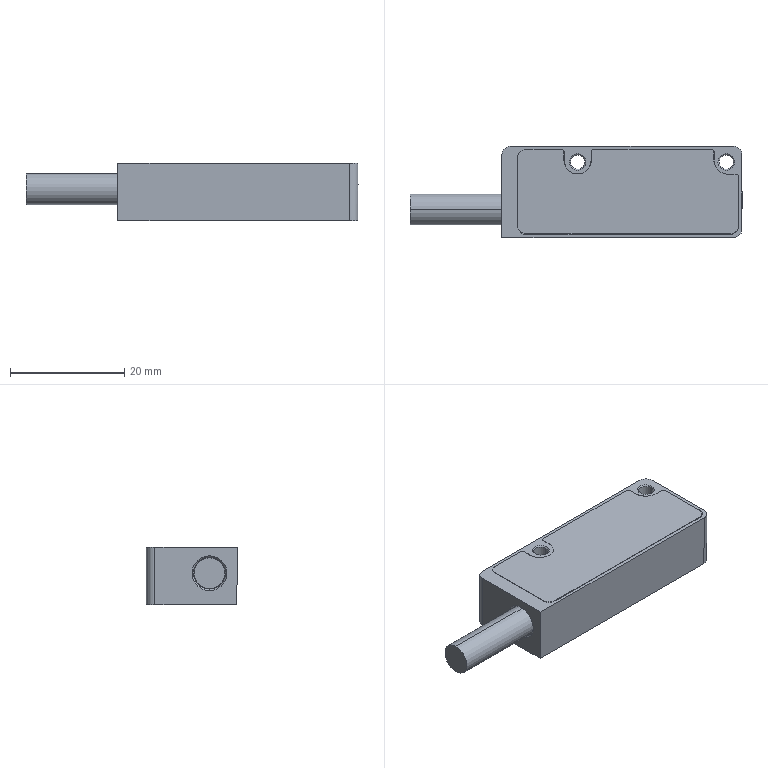Part | SolidWorks | features BaseBody 3 | 3 solids | 107 faces | box 58.084 x 15.975 x 10 mm | volume 3195 mm3 | plane 49 | cylinder 39 | cone 13 | spline 6 | commonest cylinder face diameters 1 x9 3 x8 1.6 x4 2 x4 2.5 x4 5 x3